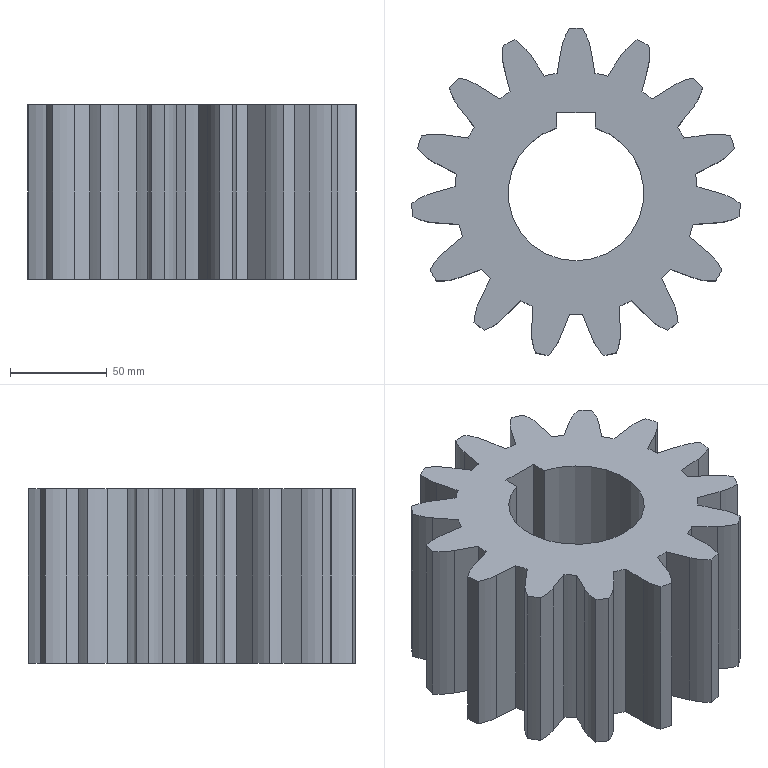Part | Creo | features PROTRUSION 16, CURVE 3, DATUM PLANE 3, COORDINATE SYSTEM 1, CUT 1, PATTERN 1 | 1 solid | 96 faces | box 169.638 x 168.774 x 90 mm | volume 1195621 mm3 | cylinder 61 | plane 35 | commonest cylinder face diameters 53.781 x30 125 x15 170 x15 70 x1